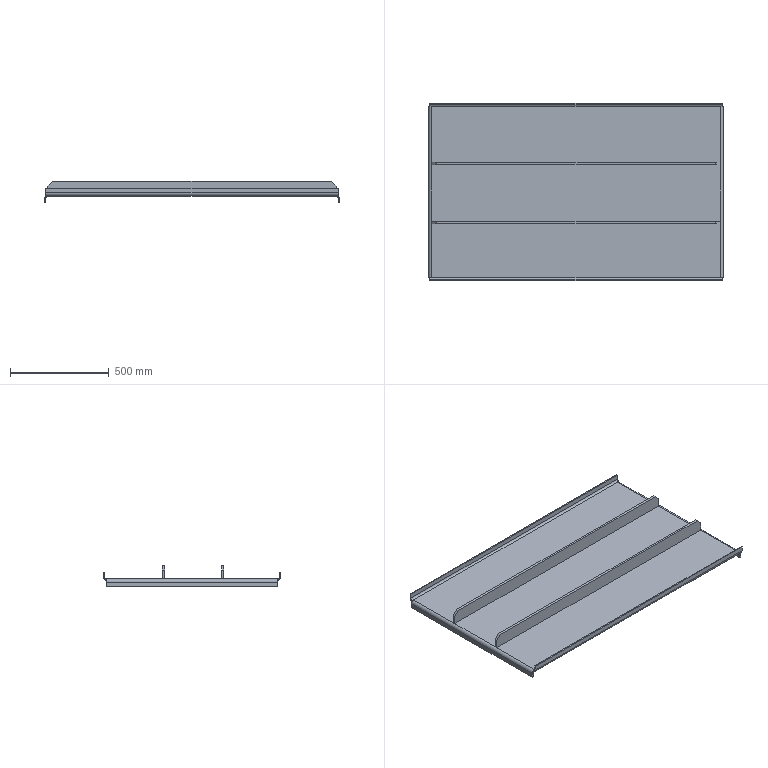Part | SolidWorks | features Chamfer 2, EdgeFlange 2, BossThin 1, FlatPattern 1, SMBaseFlange 1, SheetMetal 1, WeldmentFeature 1 | 3 solids | 58 faces | box 1492 x 898 x 110 mm | volume 11274482 mm3 | plane 50 | cylinder 8 | commonest cylinder face diameters 20 x4 32 x4
STEP:
#1=CARTESIAN_POINT('',(740.,-433.,0.));
#2=VERTEX_POINT('',#1);
#3=CARTESIAN_POINT('',(740.,-433.,-3.51));
#4=VERTEX_POINT('',#3);
#5=CARTESIAN_POINT('',(740.,-433.,0.));
#6=DIRECTION('',(0.,0.,-1.));
#7=VECTOR('',#6,1000.);
#8=LINE('',#5,#7);
#9=EDGE_CURVE('',#2,#4,#8,.T.);
#10=ORIENTED_EDGE('',*,*,#9,.T.);
#11=CARTESIAN_POINT('',(730.,-433.,0.));
#12=VERTEX_POINT('',#11);
#13=CARTESIAN_POINT('',(730.,-433.,-16.));
#14=DIRECTION('',(0.,-1.,0.));
#15=DIRECTION('',(0.,0.,-1.));
#16=AXIS2_PLACEMENT_3D('',#13,#14,#15);
#17=CIRCLE('',#16,16.);
#18=EDGE_CURVE('',#4,#12,#17,.T.);
#19=ORIENTED_EDGE('',*,*,#18,.T.);
#20=CARTESIAN_POINT('',(740.,-433.,0.));
#21=DIRECTION('',(-1.,0.,0.));
#22=VECTOR('',#21,1000.);
#23=LINE('',#20,#22);
#24=EDGE_CURVE('',#2,#12,#23,.T.);
#25=ORIENTED_EDGE('',*,*,#24,.F.);
#26=EDGE_LOOP('',(#10,#19,#25));
#27=FACE_OUTER_BOUND('',#26,.T.);
#28=CARTESIAN_POINT('',(740.,-433.,-6.));
#29=DIRECTION('',(0.,1.,0.));
#30=DIRECTION('',(0.,0.,1.));
#31=AXIS2_PLACEMENT_3D('',#28,#29,#30);
#32=PLANE('',#31);
#33=ADVANCED_FACE('',(#27),#32,.T.);
#34=CARTESIAN_POINT('',(730.,433.,0.));
#35=VERTEX_POINT('',#34);
#36=CARTESIAN_POINT('',(740.,433.,0.));
#37=VERTEX_POINT('',#36);
#38=CARTESIAN_POINT('',(-740.,433.,0.));
#39=DIRECTION('',(1.,0.,0.));
#40=VECTOR('',#39,1000.);
#41=LINE('',#38,#40);
#42=EDGE_CURVE('',#35,#37,#41,.T.);
#43=ORIENTED_EDGE('',*,*,#42,.F.);
#44=CARTESIAN_POINT('',(740.,433.,-3.51));
#45=VERTEX_POINT('',#44);
#46=CARTESIAN_POINT('',(730.,433.,-16.));
#47=DIRECTION('',(0.,1.,0.));
#48=DIRECTION('',(0.,0.,-1.));
#49=AXIS2_PLACEMENT_3D('',#46,#47,#48);
#50=CIRCLE('',#49,16.);
#51=EDGE_CURVE('',#35,#45,#50,.T.);
#52=ORIENTED_EDGE('',*,*,#51,.T.);
#53=CARTESIAN_POINT('',(740.,433.,0.));
#54=DIRECTION('',(0.,0.,-1.));
#55=VECTOR('',#54,1000.);
#56=LINE('',#53,#55);
#57=EDGE_CURVE('',#37,#45,#56,.T.);
#58=ORIENTED_EDGE('',*,*,#57,.F.);
#59=EDGE_LOOP('',(#43,#52,#58));
#60=FACE_OUTER_BOUND('',#59,.T.);
#61=CARTESIAN_POINT('',(730.,433.,-6.));
#62=DIRECTION('',(0.,-1.,0.));
#63=DIRECTION('',(1.,0.,0.));
#64=AXIS2_PLACEMENT_3D('',#61,#62,#63);
#65=PLANE('',#64);
#66=ADVANCED_FACE('',(#60),#65,.T.);
#67=CARTESIAN_POINT('',(-740.,433.,0.));
#68=VERTEX_POINT('',#67);
#69=CARTESIAN_POINT('',(-740.,433.,-3.51));
#70=VERTEX_POINT('',#69);
#71=CARTESIAN_POINT('',(-740.,433.,0.));
#72=DIRECTION('',(0.,0.,-1.));
#73=VECTOR('',#72,1000.);
#74=LINE('',#71,#73);
#75=EDGE_CURVE('',#68,#70,#74,.T.);
#76=ORIENTED_EDGE('',*,*,#75,.T.);
#77=CARTESIAN_POINT('',(-730.,433.,0.));
#78=VERTEX_POINT('',#77);
#79=CARTESIAN_POINT('',(-730.,433.,-16.));
#80=DIRECTION('',(0.,1.,0.));
#81=DIRECTION('',(0.,0.,1.));
#82=AXIS2_PLACEMENT_3D('',#79,#80,#81);
#83=CIRCLE('',#82,16.);
#84=EDGE_CURVE('',#70,#78,#83,.T.);
#85=ORIENTED_EDGE('',*,*,#84,.T.);
#86=CARTESIAN_POINT('',(-740.,433.,0.));
#87=DIRECTION('',(1.,0.,0.));
#88=VECTOR('',#87,1000.);
#89=LINE('',#86,#88);
#90=EDGE_CURVE('',#68,#78,#89,.T.);
#91=ORIENTED_EDGE('',*,*,#90,.F.);
#92=EDGE_LOOP('',(#76,#85,#91));
#93=FACE_OUTER_BOUND('',#92,.T.);
#94=CARTESIAN_POINT('',(-740.,433.,-6.));
#95=DIRECTION('',(0.,-1.,0.));
#96=DIRECTION('',(0.,0.,-1.));
#97=AXIS2_PLACEMENT_3D('',#94,#95,#96);
#98=PLANE('',#97);
#99=ADVANCED_FACE('',(#93),#98,.T.);
#100=CARTESIAN_POINT('',(-730.,-433.,0.));
#101=VERTEX_POINT('',#100);
#102=CARTESIAN_POINT('',(-740.,-433.,0.));
#103=VERTEX_POINT('',#102);
#104=CARTESIAN_POINT('',(740.,-433.,0.));
#105=DIRECTION('',(-1.,0.,0.));
#106=VECTOR('',#105,1000.);
#107=LINE('',#104,#106);
#108=EDGE_CURVE('',#101,#103,#107,.T.);
#109=ORIENTED_EDGE('',*,*,#108,.F.);
#110=CARTESIAN_POINT('',(-740.,-433.,-3.51));
#111=VERTEX_POINT('',#110);
#112=CARTESIAN_POINT('',(-730.,-433.,-16.));
#113=DIRECTION('',(0.,-1.,0.));
#114=DIRECTION('',(0.,0.,1.));
#115=AXIS2_PLACEMENT_3D('',#112,#113,#114);
#116=CIRCLE('',#115,16.);
#117=EDGE_CURVE('',#101,#111,#116,.T.);
#118=ORIENTED_EDGE('',*,*,#117,.T.);
#119=CARTESIAN_POINT('',(-740.,-433.,0.));
#120=DIRECTION('',(0.,0.,-1.));
#121=VECTOR('',#120,1000.);
#122=LINE('',#119,#121);
#123=EDGE_CURVE('',#103,#111,#122,.T.);
#124=ORIENTED_EDGE('',*,*,#123,.F.);
#125=EDGE_LOOP('',(#109,#118,#124));
#126=FACE_OUTER_BOUND('',#125,.T.);
#127=CARTESIAN_POINT('',(-730.,-433.,-6.));
#128=DIRECTION('',(0.,1.,0.));
#129=DIRECTION('',(0.,0.,1.));
#130=AXIS2_PLACEMENT_3D('',#127,#128,#129);
#131=PLANE('',#130);
#132=ADVANCED_FACE('',(#126),#131,.T.);
#133=CARTESIAN_POINT('',(730.,-433.,-6.));
#134=VERTEX_POINT('',#133);
#135=CARTESIAN_POINT('',(730.,433.,-6.));
#136=VERTEX_POINT('',#135);
#137=CARTESIAN_POINT('',(730.,-433.,-6.));
#138=DIRECTION('',(0.,1.,0.));
#139=VECTOR('',#138,1000.);
#140=LINE('',#137,#139);
#141=EDGE_CURVE('',#134,#136,#140,.T.);
#142=ORIENTED_EDGE('',*,*,#141,.F.);
#143=CARTESIAN_POINT('',(-730.,-433.,-6.));
#144=VERTEX_POINT('',#143);
#145=CARTESIAN_POINT('',(740.,-433.,-6.));
#146=DIRECTION('',(-1.,0.,0.));
#147=VECTOR('',#146,1000.);
#148=LINE('',#145,#147);
#149=EDGE_CURVE('',#134,#144,#148,.T.);
#150=ORIENTED_EDGE('',*,*,#149,.T.);
#151=CARTESIAN_POINT('',(-730.,433.,-6.));
#152=VERTEX_POINT('',#151);
#153=CARTESIAN_POINT('',(-730.,433.,-6.));
#154=DIRECTION('',(0.,-1.,0.));
#155=VECTOR('',#154,1000.);
#156=LINE('',#153,#155);
#157=EDGE_CURVE('',#152,#144,#156,.T.);
#158=ORIENTED_EDGE('',*,*,#157,.F.);
#159=CARTESIAN_POINT('',(-740.,433.,-6.));
#160=DIRECTION('',(1.,0.,0.));
#161=VECTOR('',#160,1000.);
#162=LINE('',#159,#161);
#163=EDGE_CURVE('',#152,#136,#162,.T.);
#164=ORIENTED_EDGE('',*,*,#163,.T.);
#165=EDGE_LOOP('',(#142,#150,#158,#164));
#166=FACE_OUTER_BOUND('',#165,.T.);
#167=CARTESIAN_POINT('',(0.,0.,-6.));
#168=DIRECTION('',(0.,0.,1.));
#169=DIRECTION('',(1.,0.,0.));
#170=AXIS2_PLACEMENT_3D('',#167,#168,#169);
#171=PLANE('',#170);
#172=ADVANCED_FACE('',(#166),#171,.F.);
#173=CARTESIAN_POINT('',(740.,-433.,0.));
#174=DIRECTION('',(-1.,0.,0.));
#175=VECTOR('',#174,1000.);
#176=LINE('',#173,#175);
#177=EDGE_CURVE('',#12,#101,#176,.T.);
#178=ORIENTED_EDGE('',*,*,#177,.F.);
#179=CARTESIAN_POINT('',(730.,-433.,0.));
#180=DIRECTION('',(0.,1.,0.));
#181=VECTOR('',#180,1000.);
#182=LINE('',#179,#181);
#183=EDGE_CURVE('',#12,#35,#182,.T.);
#184=ORIENTED_EDGE('',*,*,#183,.T.);
#185=CARTESIAN_POINT('',(-740.,433.,0.));
#186=DIRECTION('',(1.,0.,0.));
#187=VECTOR('',#186,1000.);
#188=LINE('',#185,#187);
#189=EDGE_CURVE('',#78,#35,#188,.T.);
#190=ORIENTED_EDGE('',*,*,#189,.F.);
#191=CARTESIAN_POINT('',(-730.,433.,0.));
#192=DIRECTION('',(0.,-1.,0.));
#193=VECTOR('',#192,1000.);
#194=LINE('',#191,#193);
#195=EDGE_CURVE('',#78,#101,#194,.T.);
#196=ORIENTED_EDGE('',*,*,#195,.T.);
#197=EDGE_LOOP('',(#178,#184,#190,#196));
#198=FACE_OUTER_BOUND('',#197,.T.);
#199=CARTESIAN_POINT('',(0.,0.,0.));
#200=DIRECTION('',(0.,0.,1.));
#201=DIRECTION('',(1.,0.,0.));
#202=AXIS2_PLACEMENT_3D('',#199,#200,#201);
#203=PLANE('',#202);
#204=ADVANCED_FACE('',(#198),#203,.T.);
#205=CARTESIAN_POINT('',(740.,443.,10.));
#206=VERTEX_POINT('',#205);
#207=CARTESIAN_POINT('',(740.,449.,10.));
#208=VERTEX_POINT('',#207);
#209=CARTESIAN_POINT('',(740.,449.,10.));
#210=DIRECTION('',(0.,1.,0.));
#211=VECTOR('',#210,1000.);
#212=LINE('',#209,#211);
#213=EDGE_CURVE('',#206,#208,#212,.T.);
#214=ORIENTED_EDGE('',*,*,#213,.F.);
#215=CARTESIAN_POINT('',(740.,433.,10.));
#216=DIRECTION('',(1.,0.,0.));
#217=DIRECTION('',(0.,0.,1.));
#218=AXIS2_PLACEMENT_3D('',#215,#216,#217);
#219=CIRCLE('',#218,10.);
#220=EDGE_CURVE('',#37,#206,#219,.T.);
#221=ORIENTED_EDGE('',*,*,#220,.F.);
#222=ORIENTED_EDGE('',*,*,#57,.T.);
#223=CARTESIAN_POINT('',(740.,433.,-6.));
#224=VERTEX_POINT('',#223);
#225=CARTESIAN_POINT('',(740.,433.,0.));
#226=DIRECTION('',(0.,0.,-1.));
#227=VECTOR('',#226,1000.);
#228=LINE('',#225,#227);
#229=EDGE_CURVE('',#45,#224,#228,.T.);
#230=ORIENTED_EDGE('',*,*,#229,.T.);
#231=CARTESIAN_POINT('',(740.,433.,10.));
#232=DIRECTION('',(1.,0.,0.));
#233=DIRECTION('',(0.,0.,1.));
#234=AXIS2_PLACEMENT_3D('',#231,#232,#233);
#235=CIRCLE('',#234,16.);
#236=EDGE_CURVE('',#224,#208,#235,.T.);
#237=ORIENTED_EDGE('',*,*,#236,.T.);
#238=EDGE_LOOP('',(#214,#221,#222,#230,#237));
#239=FACE_OUTER_BOUND('',#238,.T.);
#240=CARTESIAN_POINT('',(740.,433.,10.));
#241=DIRECTION('',(1.,0.,0.));
#242=DIRECTION('',(0.,0.,-1.));
#243=AXIS2_PLACEMENT_3D('',#240,#241,#242);
#244=PLANE('',#243);
#245=ADVANCED_FACE('',(#239),#244,.T.);
#246=CARTESIAN_POINT('',(-740.,443.,10.));
#247=VERTEX_POINT('',#246);
#248=CARTESIAN_POINT('',(-740.,433.,10.));
#249=DIRECTION('',(-1.,0.,0.));
#250=DIRECTION('',(0.,0.,1.));
#251=AXIS2_PLACEMENT_3D('',#248,#249,#250);
#252=CIRCLE('',#251,10.);
#253=EDGE_CURVE('',#247,#68,#252,.T.);
#254=ORIENTED_EDGE('',*,*,#253,.F.);
#255=CARTESIAN_POINT('',(-740.,449.,10.));
#256=VERTEX_POINT('',#255);
#257=CARTESIAN_POINT('',(-740.,443.,10.));
#258=DIRECTION('',(0.,1.,0.));
#259=VECTOR('',#258,1000.);
#260=LINE('',#257,#259);
#261=EDGE_CURVE('',#247,#256,#260,.T.);
#262=ORIENTED_EDGE('',*,*,#261,.T.);
#263=CARTESIAN_POINT('',(-740.,433.,-6.));
#264=VERTEX_POINT('',#263);
#265=CARTESIAN_POINT('',(-740.,433.,10.));
#266=DIRECTION('',(-1.,0.,0.));
#267=DIRECTION('',(0.,0.,1.));
#268=AXIS2_PLACEMENT_3D('',#265,#266,#267);
#269=CIRCLE('',#268,16.);
#270=EDGE_CURVE('',#256,#264,#269,.T.);
#271=ORIENTED_EDGE('',*,*,#270,.T.);
#272=CARTESIAN_POINT('',(-740.,433.,0.));
#273=DIRECTION('',(0.,0.,-1.));
#274=VECTOR('',#273,1000.);
#275=LINE('',#272,#274);
#276=EDGE_CURVE('',#70,#264,#275,.T.);
#277=ORIENTED_EDGE('',*,*,#276,.F.);
#278=ORIENTED_EDGE('',*,*,#75,.F.);
#279=EDGE_LOOP('',(#254,#262,#271,#277,#278));
#280=FACE_OUTER_BOUND('',#279,.T.);
#281=CARTESIAN_POINT('',(-740.,433.,10.));
#282=DIRECTION('',(1.,0.,0.));
#283=DIRECTION('',(0.,0.,-1.));
#284=AXIS2_PLACEMENT_3D('',#281,#282,#283);
#285=PLANE('',#284);
#286=ADVANCED_FACE('',(#280),#285,.F.);
#287=CARTESIAN_POINT('',(-740.,433.,-6.));
#288=DIRECTION('',(1.,0.,0.));
#289=VECTOR('',#288,1000.);
#290=LINE('',#287,#289);
#291=EDGE_CURVE('',#264,#152,#290,.T.);
#292=ORIENTED_EDGE('',*,*,#291,.F.);
#293=ORIENTED_EDGE('',*,*,#270,.F.);
#294=CARTESIAN_POINT('',(740.,449.,10.));
#295=DIRECTION('',(1.,0.,0.));
#296=VECTOR('',#295,1000.);
#297=LINE('',#294,#296);
#298=EDGE_CURVE('',#256,#208,#297,.T.);
#299=ORIENTED_EDGE('',*,*,#298,.T.);
#300=ORIENTED_EDGE('',*,*,#236,.F.);
#301=CARTESIAN_POINT('',(730.,433.,-6.));
#302=DIRECTION('',(1.,0.,0.));
#303=VECTOR('',#302,1000.);
#304=LINE('',#301,#303);
#305=EDGE_CURVE('',#136,#224,#304,.T.);
#306=ORIENTED_EDGE('',*,*,#305,.F.);
#307=ORIENTED_EDGE('',*,*,#163,.F.);
#308=EDGE_LOOP('',(#292,#293,#299,#300,#306,#307));
#309=FACE_OUTER_BOUND('',#308,.T.);
#310=CARTESIAN_POINT('',(-740.,433.,10.));
#311=DIRECTION('',(-1.,0.,0.));
#312=DIRECTION('',(0.,1.,0.));
#313=AXIS2_PLACEMENT_3D('',#310,#311,#312);
#314=CYLINDRICAL_SURFACE('',#313,16.);
#315=ADVANCED_FACE('',(#309),#314,.T.);
#316=ORIENTED_EDGE('',*,*,#90,.T.);
#317=ORIENTED_EDGE('',*,*,#189,.T.);
#318=ORIENTED_EDGE('',*,*,#42,.T.);
#319=ORIENTED_EDGE('',*,*,#220,.T.);
#320=CARTESIAN_POINT('',(740.,443.,10.));
#321=DIRECTION('',(-1.,0.,0.));
#322=VECTOR('',#321,1000.);
#323=LINE('',#320,#322);
#324=EDGE_CURVE('',#206,#247,#323,.T.);
#325=ORIENTED_EDGE('',*,*,#324,.T.);
#326=ORIENTED_EDGE('',*,*,#253,.T.);
#327=EDGE_LOOP('',(#316,#317,#318,#319,#325,#326));
#328=FACE_OUTER_BOUND('',#327,.T.);
#329=CARTESIAN_POINT('',(-740.,433.,10.));
#330=DIRECTION('',(-1.,0.,0.));
#331=DIRECTION('',(0.,1.,0.));
#332=AXIS2_PLACEMENT_3D('',#329,#330,#331);
#333=CYLINDRICAL_SURFACE('',#332,10.);
#334=ADVANCED_FACE('',(#328),#333,.F.);
#335=ORIENTED_EDGE('',*,*,#213,.T.);
#336=CARTESIAN_POINT('',(740.,449.,34.));
#337=VERTEX_POINT('',#336);
#338=CARTESIAN_POINT('',(740.,449.,0.));
#339=DIRECTION('',(0.,0.,-1.));
#340=VECTOR('',#339,1000.);
#341=LINE('',#338,#340);
#342=EDGE_CURVE('',#337,#208,#341,.T.);
#343=ORIENTED_EDGE('',*,*,#342,.F.);
#344=CARTESIAN_POINT('',(740.,443.,34.));
#345=VERTEX_POINT('',#344);
#346=CARTESIAN_POINT('',(740.,449.,34.));
#347=DIRECTION('',(0.,-1.,0.));
#348=VECTOR('',#347,1000.);
#349=LINE('',#346,#348);
#350=EDGE_CURVE('',#337,#345,#349,.T.);
#351=ORIENTED_EDGE('',*,*,#350,.T.);
#352=CARTESIAN_POINT('',(740.,443.,0.));
#353=DIRECTION('',(0.,0.,-1.));
#354=VECTOR('',#353,1000.);
#355=LINE('',#352,#354);
#356=EDGE_CURVE('',#345,#206,#355,.T.);
#357=ORIENTED_EDGE('',*,*,#356,.T.);
#358=EDGE_LOOP('',(#335,#343,#351,#357));
#359=FACE_OUTER_BOUND('',#358,.T.);
#360=CARTESIAN_POINT('',(740.,449.,0.));
#361=DIRECTION('',(-1.,0.,0.));
#362=DIRECTION('',(0.,0.,1.));
#363=AXIS2_PLACEMENT_3D('',#360,#361,#362);
#364=PLANE('',#363);
#365=ADVANCED_FACE('',(#359),#364,.F.);
#366=ORIENTED_EDGE('',*,*,#261,.F.);
#367=CARTESIAN_POINT('',(-740.,443.,34.));
#368=VERTEX_POINT('',#367);
#369=CARTESIAN_POINT('',(-740.,443.,34.));
#370=DIRECTION('',(0.,0.,1.));
#371=VECTOR('',#370,1000.);
#372=LINE('',#369,#371);
#373=EDGE_CURVE('',#247,#368,#372,.T.);
#374=ORIENTED_EDGE('',*,*,#373,.T.);
#375=CARTESIAN_POINT('',(-740.,449.,34.));
#376=VERTEX_POINT('',#375);
#377=CARTESIAN_POINT('',(-740.,449.,34.));
#378=DIRECTION('',(0.,-1.,0.));
#379=VECTOR('',#378,1000.);
#380=LINE('',#377,#379);
#381=EDGE_CURVE('',#376,#368,#380,.T.);
#382=ORIENTED_EDGE('',*,*,#381,.F.);
#383=CARTESIAN_POINT('',(-740.,449.,0.));
#384=DIRECTION('',(0.,0.,1.));
#385=VECTOR('',#384,1000.);
#386=LINE('',#383,#385);
#387=EDGE_CURVE('',#256,#376,#386,.T.);
#388=ORIENTED_EDGE('',*,*,#387,.F.);
#389=EDGE_LOOP('',(#366,#374,#382,#388));
#390=FACE_OUTER_BOUND('',#389,.T.);
#391=CARTESIAN_POINT('',(-740.,449.,34.));
#392=DIRECTION('',(1.,0.,0.));
#393=DIRECTION('',(0.,0.,-1.));
#394=AXIS2_PLACEMENT_3D('',#391,#392,#393);
#395=PLANE('',#394);
#396=ADVANCED_FACE('',(#390),#395,.F.);
#397=ORIENTED_EDGE('',*,*,#298,.F.);
#398=ORIENTED_EDGE('',*,*,#387,.T.);
#399=CARTESIAN_POINT('',(0.,449.,34.));
#400=DIRECTION('',(1.,0.,0.));
#401=VECTOR('',#400,1000.);
#402=LINE('',#399,#401);
#403=EDGE_CURVE('',#376,#337,#402,.T.);
#404=ORIENTED_EDGE('',*,*,#403,.T.);
#405=ORIENTED_EDGE('',*,*,#342,.T.);
#406=EDGE_LOOP('',(#397,#398,#404,#405));
#407=FACE_OUTER_BOUND('',#406,.T.);
#408=CARTESIAN_POINT('',(0.,449.,0.));
#409=DIRECTION('',(0.,-1.,0.));
#410=DIRECTION('',(0.,0.,-1.));
#411=AXIS2_PLACEMENT_3D('',#408,#409,#410);
#412=PLANE('',#411);
#413=ADVANCED_FACE('',(#407),#412,.F.);
#414=ORIENTED_EDGE('',*,*,#373,.F.);
#415=ORIENTED_EDGE('',*,*,#324,.F.);
#416=ORIENTED_EDGE('',*,*,#356,.F.);
#417=CARTESIAN_POINT('',(740.,443.,34.));
#418=DIRECTION('',(1.,0.,0.));
#419=VECTOR('',#418,1000.);
#420=LINE('',#417,#419);
#421=EDGE_CURVE('',#368,#345,#420,.T.);
#422=ORIENTED_EDGE('',*,*,#421,.F.);
#423=EDGE_LOOP('',(#414,#415,#416,#422));
#424=FACE_OUTER_BOUND('',#423,.T.);
#425=CARTESIAN_POINT('',(0.,443.,0.));
#426=DIRECTION('',(0.,-1.,0.));
#427=DIRECTION('',(0.,0.,-1.));
#428=AXIS2_PLACEMENT_3D('',#425,#426,#427);
#429=PLANE('',#428);
#430=ADVANCED_FACE('',(#424),#429,.T.);
#431=ORIENTED_EDGE('',*,*,#421,.T.);
#432=ORIENTED_EDGE('',*,*,#350,.F.);
#433=ORIENTED_EDGE('',*,*,#403,.F.);
#434=ORIENTED_EDGE('',*,*,#381,.T.);
#435=EDGE_LOOP('',(#431,#432,#433,#434));
#436=FACE_OUTER_BOUND('',#435,.T.);
#437=CARTESIAN_POINT('',(740.,449.,34.));
#438=DIRECTION('',(0.,0.,-1.));
#439=DIRECTION('',(0.,1.,0.));
#440=AXIS2_PLACEMENT_3D('',#437,#438,#439);
#441=PLANE('',#440);
#442=ADVANCED_FACE('',(#436),#441,.F.);
#443=CARTESIAN_POINT('',(-740.,-443.,10.));
#444=VERTEX_POINT('',#443);
#445=CARTESIAN_POINT('',(-740.,-449.,10.));
#446=VERTEX_POINT('',#445);
#447=CARTESIAN_POINT('',(-740.,-449.,10.));
#448=DIRECTION('',(0.,-1.,0.));
#449=VECTOR('',#448,1000.);
#450=LINE('',#447,#449);
#451=EDGE_CURVE('',#444,#446,#450,.T.);
#452=ORIENTED_EDGE('',*,*,#451,.F.);
#453=CARTESIAN_POINT('',(-740.,-433.,10.));
#454=DIRECTION('',(-1.,0.,0.));
#455=DIRECTION('',(0.,0.,-1.));
#456=AXIS2_PLACEMENT_3D('',#453,#454,#455);
#457=CIRCLE('',#456,10.);
#458=EDGE_CURVE('',#103,#444,#457,.T.);
#459=ORIENTED_EDGE('',*,*,#458,.F.);
#460=ORIENTED_EDGE('',*,*,#123,.T.);
#461=CARTESIAN_POINT('',(-740.,-433.,-6.));
#462=VERTEX_POINT('',#461);
#463=CARTESIAN_POINT('',(-740.,-433.,0.));
#464=DIRECTION('',(0.,0.,-1.));
#465=VECTOR('',#464,1000.);
#466=LINE('',#463,#465);
#467=EDGE_CURVE('',#111,#462,#466,.T.);
#468=ORIENTED_EDGE('',*,*,#467,.T.);
#469=CARTESIAN_POINT('',(-740.,-433.,10.));
#470=DIRECTION('',(-1.,0.,0.));
#471=DIRECTION('',(0.,0.,-1.));
#472=AXIS2_PLACEMENT_3D('',#469,#470,#471);
#473=CIRCLE('',#472,16.);
#474=EDGE_CURVE('',#462,#446,#473,.T.);
#475=ORIENTED_EDGE('',*,*,#474,.T.);
#476=EDGE_LOOP('',(#452,#459,#460,#468,#475));
#477=FACE_OUTER_BOUND('',#476,.T.);
#478=CARTESIAN_POINT('',(-740.,-433.,10.));
#479=DIRECTION('',(-1.,0.,0.));
#480=DIRECTION('',(0.,0.,1.));
#481=AXIS2_PLACEMENT_3D('',#478,#479,#480);
#482=PLANE('',#481);
#483=ADVANCED_FACE('',(#477),#482,.T.);
#484=CARTESIAN_POINT('',(740.,-443.,10.));
#485=VERTEX_POINT('',#484);
#486=CARTESIAN_POINT('',(740.,-433.,10.));
#487=DIRECTION('',(1.,0.,0.));
#488=DIRECTION('',(0.,0.,-1.));
#489=AXIS2_PLACEMENT_3D('',#486,#487,#488);
#490=CIRCLE('',#489,10.);
#491=EDGE_CURVE('',#485,#2,#490,.T.);
#492=ORIENTED_EDGE('',*,*,#491,.F.);
#493=CARTESIAN_POINT('',(740.,-449.,10.));
#494=VERTEX_POINT('',#493);
#495=CARTESIAN_POINT('',(740.,-443.,10.));
#496=DIRECTION('',(0.,-1.,0.));
#497=VECTOR('',#496,1000.);
#498=LINE('',#495,#497);
#499=EDGE_CURVE('',#485,#494,#498,.T.);
#500=ORIENTED_EDGE('',*,*,#499,.T.);
#501=CARTESIAN_POINT('',(740.,-433.,-6.));
#502=VERTEX_POINT('',#501);
#503=CARTESIAN_POINT('',(740.,-433.,10.));
#504=DIRECTION('',(1.,0.,0.));
#505=DIRECTION('',(0.,0.,-1.));
#506=AXIS2_PLACEMENT_3D('',#503,#504,#505);
#507=CIRCLE('',#506,16.);
#508=EDGE_CURVE('',#494,#502,#507,.T.);
#509=ORIENTED_EDGE('',*,*,#508,.T.);
#510=CARTESIAN_POINT('',(740.,-433.,0.));
#511=DIRECTION('',(0.,0.,-1.));
#512=VECTOR('',#511,1000.);
#513=LINE('',#510,#512);
#514=EDGE_CURVE('',#4,#502,#513,.T.);
#515=ORIENTED_EDGE('',*,*,#514,.F.);
#516=ORIENTED_EDGE('',*,*,#9,.F.);
#517=EDGE_LOOP('',(#492,#500,#509,#515,#516));
#518=FACE_OUTER_BOUND('',#517,.T.);
#519=CARTESIAN_POINT('',(740.,-433.,10.));
#520=DIRECTION('',(-1.,0.,0.));
#521=DIRECTION('',(0.,0.,1.));
#522=AXIS2_PLACEMENT_3D('',#519,#520,#521);
#523=PLANE('',#522);
#524=ADVANCED_FACE('',(#518),#523,.F.);
#525=CARTESIAN_POINT('',(740.,-433.,-6.));
#526=DIRECTION('',(-1.,0.,0.));
#527=VECTOR('',#526,1000.);
#528=LINE('',#525,#527);
#529=EDGE_CURVE('',#502,#134,#528,.T.);
#530=ORIENTED_EDGE('',*,*,#529,.F.);
#531=ORIENTED_EDGE('',*,*,#508,.F.);
#532=CARTESIAN_POINT('',(-740.,-449.,10.));
#533=DIRECTION('',(-1.,0.,0.));
#534=VECTOR('',#533,1000.);
#535=LINE('',#532,#534);
#536=EDGE_CURVE('',#494,#446,#535,.T.);
#537=ORIENTED_EDGE('',*,*,#536,.T.);
#538=ORIENTED_EDGE('',*,*,#474,.F.);
#539=CARTESIAN_POINT('',(-730.,-433.,-6.));
#540=DIRECTION('',(-1.,0.,0.));
#541=VECTOR('',#540,1000.);
#542=LINE('',#539,#541);
#543=EDGE_CURVE('',#144,#462,#542,.T.);
#544=ORIENTED_EDGE('',*,*,#543,.F.);
#545=ORIENTED_EDGE('',*,*,#149,.F.);
#546=EDGE_LOOP('',(#530,#531,#537,#538,#544,#545));
#547=FACE_OUTER_BOUND('',#546,.T.);
#548=CARTESIAN_POINT('',(740.,-433.,10.));
#549=DIRECTION('',(1.,0.,0.));
#550=DIRECTION('',(0.,-1.,0.));
#551=AXIS2_PLACEMENT_3D('',#548,#549,#550);
#552=CYLINDRICAL_SURFACE('',#551,16.);
#553=ADVANCED_FACE('',(#547),#552,.T.);
#554=ORIENTED_EDGE('',*,*,#24,.T.);
#555=ORIENTED_EDGE('',*,*,#177,.T.);
#556=ORIENTED_EDGE('',*,*,#108,.T.);
#557=ORIENTED_EDGE('',*,*,#458,.T.);
#558=CARTESIAN_POINT('',(-740.,-443.,10.));
#559=DIRECTION('',(1.,0.,0.));
#560=VECTOR('',#559,1000.);
#561=LINE('',#558,#560);
#562=EDGE_CURVE('',#444,#485,#561,.T.);
#563=ORIENTED_EDGE('',*,*,#562,.T.);
#564=ORIENTED_EDGE('',*,*,#491,.T.);
#565=EDGE_LOOP('',(#554,#555,#556,#557,#563,#564));
#566=FACE_OUTER_BOUND('',#565,.T.);
#567=CARTESIAN_POINT('',(740.,-433.,10.));
#568=DIRECTION('',(1.,0.,0.));
#569=DIRECTION('',(0.,-1.,0.));
#570=AXIS2_PLACEMENT_3D('',#567,#568,#569);
#571=CYLINDRICAL_SURFACE('',#570,10.);
#572=ADVANCED_FACE('',(#566),#571,.F.);
#573=ORIENTED_EDGE('',*,*,#451,.T.);
#574=CARTESIAN_POINT('',(-740.,-449.,34.));
#575=VERTEX_POINT('',#574);
#576=CARTESIAN_POINT('',(-740.,-449.,0.));
#577=DIRECTION('',(0.,0.,-1.));
#578=VECTOR('',#577,1000.);
#579=LINE('',#576,#578);
#580=EDGE_CURVE('',#575,#446,#579,.T.);
#581=ORIENTED_EDGE('',*,*,#580,.F.);
#582=CARTESIAN_POINT('',(-740.,-443.,34.));
#583=VERTEX_POINT('',#582);
#584=CARTESIAN_POINT('',(-740.,-449.,34.));
#585=DIRECTION('',(0.,1.,0.));
#586=VECTOR('',#585,1000.);
#587=LINE('',#584,#586);
#588=EDGE_CURVE('',#575,#583,#587,.T.);
#589=ORIENTED_EDGE('',*,*,#588,.T.);
#590=CARTESIAN_POINT('',(-740.,-443.,0.));
#591=DIRECTION('',(0.,0.,-1.));
#592=VECTOR('',#591,1000.);
#593=LINE('',#590,#592);
#594=EDGE_CURVE('',#583,#444,#593,.T.);
#595=ORIENTED_EDGE('',*,*,#594,.T.);
#596=EDGE_LOOP('',(#573,#581,#589,#595));
#597=FACE_OUTER_BOUND('',#596,.T.);
#598=CARTESIAN_POINT('',(-740.,-449.,0.));
#599=DIRECTION('',(1.,0.,0.));
#600=DIRECTION('',(0.,0.,-1.));
#601=AXIS2_PLACEMENT_3D('',#598,#599,#600);
#602=PLANE('',#601);
#603=ADVANCED_FACE('',(#597),#602,.F.);
#604=ORIENTED_EDGE('',*,*,#499,.F.);
#605=CARTESIAN_POINT('',(740.,-443.,34.));
#606=VERTEX_POINT('',#605);
#607=CARTESIAN_POINT('',(740.,-443.,34.));
#608=DIRECTION('',(0.,0.,1.));
#609=VECTOR('',#608,1000.);
#610=LINE('',#607,#609);
#611=EDGE_CURVE('',#485,#606,#610,.T.);
#612=ORIENTED_EDGE('',*,*,#611,.T.);
#613=CARTESIAN_POINT('',(740.,-449.,34.));
#614=VERTEX_POINT('',#613);
#615=CARTESIAN_POINT('',(740.,-449.,34.));
#616=DIRECTION('',(0.,1.,0.));
#617=VECTOR('',#616,1000.);
#618=LINE('',#615,#617);
#619=EDGE_CURVE('',#614,#606,#618,.T.);
#620=ORIENTED_EDGE('',*,*,#619,.F.);
#621=CARTESIAN_POINT('',(740.,-449.,0.));
#622=DIRECTION('',(0.,0.,1.));
#623=VECTOR('',#622,1000.);
#624=LINE('',#621,#623);
#625=EDGE_CURVE('',#494,#614,#624,.T.);
#626=ORIENTED_EDGE('',*,*,#625,.F.);
#627=EDGE_LOOP('',(#604,#612,#620,#626));
#628=FACE_OUTER_BOUND('',#627,.T.);
#629=CARTESIAN_POINT('',(740.,-449.,34.));
#630=DIRECTION('',(-1.,0.,0.));
#631=DIRECTION('',(0.,0.,1.));
#632=AXIS2_PLACEMENT_3D('',#629,#630,#631);
#633=PLANE('',#632);
#634=ADVANCED_FACE('',(#628),#633,.F.);
#635=ORIENTED_EDGE('',*,*,#536,.F.);
#636=ORIENTED_EDGE('',*,*,#625,.T.);
#637=CARTESIAN_POINT('',(0.,-449.,34.));
#638=DIRECTION('',(-1.,0.,0.));
#639=VECTOR('',#638,1000.);
#640=LINE('',#637,#639);
#641=EDGE_CURVE('',#614,#575,#640,.T.);
#642=ORIENTED_EDGE('',*,*,#641,.T.);
#643=ORIENTED_EDGE('',*,*,#580,.T.);
#644=EDGE_LOOP('',(#635,#636,#642,#643));
#645=FACE_OUTER_BOUND('',#644,.T.);
#646=CARTESIAN_POINT('',(0.,-449.,0.));
#647=DIRECTION('',(0.,1.,0.));
#648=DIRECTION('',(0.,0.,1.));
#649=AXIS2_PLACEMENT_3D('',#646,#647,#648);
#650=PLANE('',#649);
#651=ADVANCED_FACE('',(#645),#650,.F.);
#652=ORIENTED_EDGE('',*,*,#611,.F.);
#653=ORIENTED_EDGE('',*,*,#562,.F.);
#654=ORIENTED_EDGE('',*,*,#594,.F.);
#655=CARTESIAN_POINT('',(-740.,-443.,34.));
#656=DIRECTION('',(-1.,0.,0.));
#657=VECTOR('',#656,1000.);
#658=LINE('',#655,#657);
#659=EDGE_CURVE('',#606,#583,#658,.T.);
#660=ORIENTED_EDGE('',*,*,#659,.F.);
#661=EDGE_LOOP('',(#652,#653,#654,#660));
#662=FACE_OUTER_BOUND('',#661,.T.);
#663=CARTESIAN_POINT('',(0.,-443.,0.));
#664=DIRECTION('',(0.,1.,0.));
#665=DIRECTION('',(0.,0.,1.));
#666=AXIS2_PLACEMENT_3D('',#663,#664,#665);
#667=PLANE('',#666);
#668=ADVANCED_FACE('',(#662),#667,.T.);
#669=ORIENTED_EDGE('',*,*,#659,.T.);
#670=ORIENTED_EDGE('',*,*,#588,.F.);
#671=ORIENTED_EDGE('',*,*,#641,.F.);
#672=ORIENTED_EDGE('',*,*,#619,.T.);
#673=EDGE_LOOP('',(#669,#670,#671,#672));
#674=FACE_OUTER_BOUND('',#673,.T.);
#675=CARTESIAN_POINT('',(-740.,-449.,34.));
#676=DIRECTION('',(0.,0.,-1.));
#677=DIRECTION('',(0.,1.,0.));
#678=AXIS2_PLACEMENT_3D('',#675,#676,#677);
#679=PLANE('',#678);
#680=ADVANCED_FACE('',(#674),#679,.F.);
#681=ORIENTED_EDGE('',*,*,#467,.F.);
#682=CARTESIAN_POINT('',(-746.,-433.,-16.));
#683=VERTEX_POINT('',#682);
#684=CARTESIAN_POINT('',(-730.,-433.,-16.));
#685=DIRECTION('',(0.,-1.,0.));
#686=DIRECTION('',(0.,0.,1.));
#687=AXIS2_PLACEMENT_3D('',#684,#685,#686);
#688=CIRCLE('',#687,16.);
#689=EDGE_CURVE('',#111,#683,#688,.T.);
#690=ORIENTED_EDGE('',*,*,#689,.T.);
#691=CARTESIAN_POINT('',(-740.,-433.,-16.));
#692=VERTEX_POINT('',#691);
#693=CARTESIAN_POINT('',(-740.,-433.,-16.));
#694=DIRECTION('',(-1.,0.,0.));
#695=VECTOR('',#694,1000.);
#696=LINE('',#693,#695);
#697=EDGE_CURVE('',#692,#683,#696,.T.);
#698=ORIENTED_EDGE('',*,*,#697,.F.);
#699=CARTESIAN_POINT('',(-730.,-433.,-16.));
#700=DIRECTION('',(0.,-1.,0.));
#701=DIRECTION('',(0.,0.,1.));
#702=AXIS2_PLACEMENT_3D('',#699,#700,#701);
#703=CIRCLE('',#702,10.);
#704=EDGE_CURVE('',#144,#692,#703,.T.);
#705=ORIENTED_EDGE('',*,*,#704,.F.);
#706=ORIENTED_EDGE('',*,*,#543,.T.);
#707=EDGE_LOOP('',(#681,#690,#698,#705,#706));
#708=FACE_OUTER_BOUND('',#707,.T.);
#709=CARTESIAN_POINT('',(-730.,-433.,-16.));
#710=DIRECTION('',(0.,-1.,0.));
#711=DIRECTION('',(0.,0.,-1.));
#712=AXIS2_PLACEMENT_3D('',#709,#710,#711);
#713=PLANE('',#712);
#714=ADVANCED_FACE('',(#708),#713,.T.);
#715=CARTESIAN_POINT('',(-746.,433.,-16.));
#716=VERTEX_POINT('',#715);
#717=CARTESIAN_POINT('',(-730.,433.,-16.));
#718=DIRECTION('',(0.,1.,0.));
#719=DIRECTION('',(0.,0.,1.));
#720=AXIS2_PLACEMENT_3D('',#717,#718,#719);
#721=CIRCLE('',#720,16.);
#722=EDGE_CURVE('',#716,#70,#721,.T.);
#723=ORIENTED_EDGE('',*,*,#722,.T.);
#724=ORIENTED_EDGE('',*,*,#276,.T.);
#725=ORIENTED_EDGE('',*,*,#291,.T.);
#726=CARTESIAN_POINT('',(-740.,433.,-16.));
#727=VERTEX_POINT('',#726);
#728=CARTESIAN_POINT('',(-730.,433.,-16.));
#729=DIRECTION('',(0.,1.,0.));
#730=DIRECTION('',(0.,0.,1.));
#731=AXIS2_PLACEMENT_3D('',#728,#729,#730);
#732=CIRCLE('',#731,10.);
#733=EDGE_CURVE('',#727,#152,#732,.T.);
#734=ORIENTED_EDGE('',*,*,#733,.F.);
#735=CARTESIAN_POINT('',(-740.,433.,-16.));
#736=DIRECTION('',(-1.,0.,0.));
#737=VECTOR('',#736,1000.);
#738=LINE('',#735,#737);
#739=EDGE_CURVE('',#727,#716,#738,.T.);
#740=ORIENTED_EDGE('',*,*,#739,.T.);
#741=EDGE_LOOP('',(#723,#724,#725,#734,#740));
#742=FACE_OUTER_BOUND('',#741,.T.);
#743=CARTESIAN_POINT('',(-730.,433.,-16.));
#744=DIRECTION('',(0.,-1.,0.));
#745=DIRECTION('',(0.,0.,-1.));
#746=AXIS2_PLACEMENT_3D('',#743,#744,#745);
#747=PLANE('',#746);
#748=ADVANCED_FACE('',(#742),#747,.F.);
#749=ORIENTED_EDGE('',*,*,#195,.F.);
#750=ORIENTED_EDGE('',*,*,#84,.F.);
#751=ORIENTED_EDGE('',*,*,#722,.F.);
#752=CARTESIAN_POINT('',(-746.,0.,-16.));
#753=DIRECTION('',(0.,1.,0.));
#754=VECTOR('',#753,1000.);
#755=LINE('',#752,#754);
#756=EDGE_CURVE('',#683,#716,#755,.T.);
#757=ORIENTED_EDGE('',*,*,#756,.F.);
#758=ORIENTED_EDGE('',*,*,#689,.F.);
#759=ORIENTED_EDGE('',*,*,#117,.F.);
#760=EDGE_LOOP('',(#749,#750,#751,#757,#758,#759));
#761=FACE_OUTER_BOUND('',#760,.T.);
#762=CARTESIAN_POINT('',(-730.,433.,-16.));
#763=DIRECTION('',(0.,1.,0.));
#764=DIRECTION('',(-1.,0.,0.));
#765=AXIS2_PLACEMENT_3D('',#762,#763,#764);
#766=CYLINDRICAL_SURFACE('',#765,16.);
#767=ADVANCED_FACE('',(#761),#766,.T.);
#768=ORIENTED_EDGE('',*,*,#157,.T.);
#769=ORIENTED_EDGE('',*,*,#704,.T.);
#770=CARTESIAN_POINT('',(-740.,-433.,-16.));
#771=DIRECTION('',(0.,1.,0.));
#772=VECTOR('',#771,1000.);
#773=LINE('',#770,#772);
#774=EDGE_CURVE('',#692,#727,#773,.T.);
#775=ORIENTED_EDGE('',*,*,#774,.T.);
#776=ORIENTED_EDGE('',*,*,#733,.T.);
#777=EDGE_LOOP('',(#768,#769,#775,#776));
#778=FACE_OUTER_BOUND('',#777,.T.);
#779=CARTESIAN_POINT('',(-730.,433.,-16.));
#780=DIRECTION('',(0.,1.,0.));
#781=DIRECTION('',(-1.,0.,0.));
#782=AXIS2_PLACEMENT_3D('',#779,#780,#781);
#783=CYLINDRICAL_SURFACE('',#782,10.);
#784=ADVANCED_FACE('',(#778),#783,.F.);
#785=CARTESIAN_POINT('',(-746.,433.,-40.));
#786=VERTEX_POINT('',#785);
#787=CARTESIAN_POINT('',(-746.,433.,-6.));
#788=DIRECTION('',(0.,0.,1.));
#789=VECTOR('',#788,1000.);
#790=LINE('',#787,#789);
#791=EDGE_CURVE('',#786,#716,#790,.T.);
#792=ORIENTED_EDGE('',*,*,#791,.T.);
#793=ORIENTED_EDGE('',*,*,#739,.F.);
#794=CARTESIAN_POINT('',(-740.,433.,-40.));
#795=VERTEX_POINT('',#794);
#796=CARTESIAN_POINT('',(-740.,433.,-6.));
#797=DIRECTION('',(0.,0.,1.));
#798=VECTOR('',#797,1000.);
#799=LINE('',#796,#798);
#800=EDGE_CURVE('',#795,#727,#799,.T.);
#801=ORIENTED_EDGE('',*,*,#800,.F.);
#802=CARTESIAN_POINT('',(-746.,433.,-40.));
#803=DIRECTION('',(1.,0.,0.));
#804=VECTOR('',#803,1000.);
#805=LINE('',#802,#804);
#806=EDGE_CURVE('',#786,#795,#805,.T.);
#807=ORIENTED_EDGE('',*,*,#806,.F.);
#808=EDGE_LOOP('',(#792,#793,#801,#807));
#809=FACE_OUTER_BOUND('',#808,.T.);
#810=CARTESIAN_POINT('',(-746.,433.,-6.));
#811=DIRECTION('',(0.,1.,0.));
#812=DIRECTION('',(-1.,0.,0.));
#813=AXIS2_PLACEMENT_3D('',#810,#811,#812);
#814=PLANE('',#813);
#815=ADVANCED_FACE('',(#809),#814,.T.);
#816=CARTESIAN_POINT('',(-740.,-433.,-40.));
#817=VERTEX_POINT('',#816);
#818=CARTESIAN_POINT('',(-740.,-433.,-40.));
#819=DIRECTION('',(0.,0.,-1.));
#820=VECTOR('',#819,1000.);
#821=LINE('',#818,#820);
#822=EDGE_CURVE('',#692,#817,#821,.T.);
#823=ORIENTED_EDGE('',*,*,#822,.F.);
#824=ORIENTED_EDGE('',*,*,#697,.T.);
#825=CARTESIAN_POINT('',(-746.,-433.,-40.));
#826=VERTEX_POINT('',#825);
#827=CARTESIAN_POINT('',(-746.,-433.,-40.));
#828=DIRECTION('',(0.,0.,-1.));
#829=VECTOR('',#828,1000.);
#830=LINE('',#827,#829);
#831=EDGE_CURVE('',#683,#826,#830,.T.);
#832=ORIENTED_EDGE('',*,*,#831,.T.);
#833=CARTESIAN_POINT('',(-746.,-433.,-40.));
#834=DIRECTION('',(1.,0.,0.));
#835=VECTOR('',#834,1000.);
#836=LINE('',#833,#835);
#837=EDGE_CURVE('',#826,#817,#836,.T.);
#838=ORIENTED_EDGE('',*,*,#837,.T.);
#839=EDGE_LOOP('',(#823,#824,#832,#838));
#840=FACE_OUTER_BOUND('',#839,.T.);
#841=CARTESIAN_POINT('',(-746.,-433.,-40.));
#842=DIRECTION('',(0.,-1.,0.));
#843=DIRECTION('',(1.,0.,0.));
#844=AXIS2_PLACEMENT_3D('',#841,#842,#843);
#845=PLANE('',#844);
#846=ADVANCED_FACE('',(#840),#845,.T.);
#847=ORIENTED_EDGE('',*,*,#831,.F.);
#848=ORIENTED_EDGE('',*,*,#756,.T.);
#849=ORIENTED_EDGE('',*,*,#791,.F.);
#850=CARTESIAN_POINT('',(-746.,433.,-40.));
#851=DIRECTION('',(0.,1.,0.));
#852=VECTOR('',#851,1000.);
#853=LINE('',#850,#852);
#854=EDGE_CURVE('',#826,#786,#853,.T.);
#855=ORIENTED_EDGE('',*,*,#854,.F.);
#856=EDGE_LOOP('',(#847,#848,#849,#855));
#857=FACE_OUTER_BOUND('',#856,.T.);
#858=CARTESIAN_POINT('',(-746.,0.,0.));
#859=DIRECTION('',(-1.,0.,0.));
#860=DIRECTION('',(0.,0.,1.));
#861=AXIS2_PLACEMENT_3D('',#858,#859,#860);
#862=PLANE('',#861);
#863=ADVANCED_FACE('',(#857),#862,.T.);
#864=ORIENTED_EDGE('',*,*,#774,.F.);
#865=ORIENTED_EDGE('',*,*,#822,.T.);
#866=CARTESIAN_POINT('',(-740.,433.,-40.));
#867=DIRECTION('',(0.,1.,0.));
#868=VECTOR('',#867,1000.);
#869=LINE('',#866,#868);
#870=EDGE_CURVE('',#817,#795,#869,.T.);
#871=ORIENTED_EDGE('',*,*,#870,.T.);
#872=ORIENTED_EDGE('',*,*,#800,.T.);
#873=EDGE_LOOP('',(#864,#865,#871,#872));
#874=FACE_OUTER_BOUND('',#873,.T.);
#875=CARTESIAN_POINT('',(-740.,0.,0.));
#876=DIRECTION('',(-1.,0.,0.));
#877=DIRECTION('',(0.,0.,1.));
#878=AXIS2_PLACEMENT_3D('',#875,#876,#877);
#879=PLANE('',#878);
#880=ADVANCED_FACE('',(#874),#879,.F.);
#881=ORIENTED_EDGE('',*,*,#870,.F.);
#882=ORIENTED_EDGE('',*,*,#837,.F.);
#883=ORIENTED_EDGE('',*,*,#854,.T.);
#884=ORIENTED_EDGE('',*,*,#806,.T.);
#885=EDGE_LOOP('',(#881,#882,#883,#884));
#886=FACE_OUTER_BOUND('',#885,.T.);
#887=CARTESIAN_POINT('',(-746.,433.,-40.));
#888=DIRECTION('',(0.,0.,-1.));
#889=DIRECTION('',(-1.,0.,0.));
#890=AXIS2_PLACEMENT_3D('',#887,#888,#889);
#891=PLANE('',#890);
#892=ADVANCED_FACE('',(#886),#891,.T.);
#893=ORIENTED_EDGE('',*,*,#229,.F.);
#894=CARTESIAN_POINT('',(746.,433.,-16.));
#895=VERTEX_POINT('',#894);
#896=CARTESIAN_POINT('',(730.,433.,-16.));
#897=DIRECTION('',(0.,1.,0.));
#898=DIRECTION('',(0.,0.,-1.));
#899=AXIS2_PLACEMENT_3D('',#896,#897,#898);
#900=CIRCLE('',#899,16.);
#901=EDGE_CURVE('',#45,#895,#900,.T.);
#902=ORIENTED_EDGE('',*,*,#901,.T.);
#903=CARTESIAN_POINT('',(740.,433.,-16.));
#904=VERTEX_POINT('',#903);
#905=CARTESIAN_POINT('',(740.,433.,-16.));
#906=DIRECTION('',(1.,0.,0.));
#907=VECTOR('',#906,1000.);
#908=LINE('',#905,#907);
#909=EDGE_CURVE('',#904,#895,#908,.T.);
#910=ORIENTED_EDGE('',*,*,#909,.F.);
#911=CARTESIAN_POINT('',(730.,433.,-16.));
#912=DIRECTION('',(0.,1.,0.));
#913=DIRECTION('',(0.,0.,-1.));
#914=AXIS2_PLACEMENT_3D('',#911,#912,#913);
#915=CIRCLE('',#914,10.);
#916=EDGE_CURVE('',#136,#904,#915,.T.);
#917=ORIENTED_EDGE('',*,*,#916,.F.);
#918=ORIENTED_EDGE('',*,*,#305,.T.);
#919=EDGE_LOOP('',(#893,#902,#910,#917,#918));
#920=FACE_OUTER_BOUND('',#919,.T.);
#921=CARTESIAN_POINT('',(730.,433.,-16.));
#922=DIRECTION('',(0.,1.,0.));
#923=DIRECTION('',(0.,0.,1.));
#924=AXIS2_PLACEMENT_3D('',#921,#922,#923);
#925=PLANE('',#924);
#926=ADVANCED_FACE('',(#920),#925,.T.);
#927=CARTESIAN_POINT('',(746.,-433.,-16.));
#928=VERTEX_POINT('',#927);
#929=CARTESIAN_POINT('',(730.,-433.,-16.));
#930=DIRECTION('',(0.,-1.,0.));
#931=DIRECTION('',(0.,0.,-1.));
#932=AXIS2_PLACEMENT_3D('',#929,#930,#931);
#933=CIRCLE('',#932,16.);
#934=EDGE_CURVE('',#928,#4,#933,.T.);
#935=ORIENTED_EDGE('',*,*,#934,.T.);
#936=ORIENTED_EDGE('',*,*,#514,.T.);
#937=ORIENTED_EDGE('',*,*,#529,.T.);
#938=CARTESIAN_POINT('',(740.,-433.,-16.));
#939=VERTEX_POINT('',#938);
#940=CARTESIAN_POINT('',(730.,-433.,-16.));
#941=DIRECTION('',(0.,-1.,0.));
#942=DIRECTION('',(0.,0.,-1.));
#943=AXIS2_PLACEMENT_3D('',#940,#941,#942);
#944=CIRCLE('',#943,10.);
#945=EDGE_CURVE('',#939,#134,#944,.T.);
#946=ORIENTED_EDGE('',*,*,#945,.F.);
#947=CARTESIAN_POINT('',(740.,-433.,-16.));
#948=DIRECTION('',(1.,0.,0.));
#949=VECTOR('',#948,1000.);
#950=LINE('',#947,#949);
#951=EDGE_CURVE('',#939,#928,#950,.T.);
#952=ORIENTED_EDGE('',*,*,#951,.T.);
#953=EDGE_LOOP('',(#935,#936,#937,#946,#952));
#954=FACE_OUTER_BOUND('',#953,.T.);
#955=CARTESIAN_POINT('',(730.,-433.,-16.));
#956=DIRECTION('',(0.,1.,0.));
#957=DIRECTION('',(0.,0.,1.));
#958=AXIS2_PLACEMENT_3D('',#955,#956,#957);
#959=PLANE('',#958);
#960=ADVANCED_FACE('',(#954),#959,.F.);
#961=ORIENTED_EDGE('',*,*,#183,.F.);
#962=ORIENTED_EDGE('',*,*,#18,.F.);
#963=ORIENTED_EDGE('',*,*,#934,.F.);
#964=CARTESIAN_POINT('',(746.,0.,-16.));
#965=DIRECTION('',(0.,1.,0.));
#966=VECTOR('',#965,1000.);
#967=LINE('',#964,#966);
#968=EDGE_CURVE('',#928,#895,#967,.T.);
#969=ORIENTED_EDGE('',*,*,#968,.T.);
#970=ORIENTED_EDGE('',*,*,#901,.F.);
#971=ORIENTED_EDGE('',*,*,#51,.F.);
#972=EDGE_LOOP('',(#961,#962,#963,#969,#970,#971));
#973=FACE_OUTER_BOUND('',#972,.T.);
#974=CARTESIAN_POINT('',(730.,-433.,-16.));
#975=DIRECTION('',(0.,-1.,0.));
#976=DIRECTION('',(1.,0.,0.));
#977=AXIS2_PLACEMENT_3D('',#974,#975,#976);
#978=CYLINDRICAL_SURFACE('',#977,16.);
#979=ADVANCED_FACE('',(#973),#978,.T.);
#980=ORIENTED_EDGE('',*,*,#141,.T.);
#981=ORIENTED_EDGE('',*,*,#916,.T.);
#982=CARTESIAN_POINT('',(740.,433.,-16.));
#983=DIRECTION('',(0.,-1.,0.));
#984=VECTOR('',#983,1000.);
#985=LINE('',#982,#984);
#986=EDGE_CURVE('',#904,#939,#985,.T.);
#987=ORIENTED_EDGE('',*,*,#986,.T.);
#988=ORIENTED_EDGE('',*,*,#945,.T.);
#989=EDGE_LOOP('',(#980,#981,#987,#988));
#990=FACE_OUTER_BOUND('',#989,.T.);
#991=CARTESIAN_POINT('',(730.,-433.,-16.));
#992=DIRECTION('',(0.,-1.,0.));
#993=DIRECTION('',(1.,0.,0.));
#994=AXIS2_PLACEMENT_3D('',#991,#992,#993);
#995=CYLINDRICAL_SURFACE('',#994,10.);
#996=ADVANCED_FACE('',(#990),#995,.F.);
#997=CARTESIAN_POINT('',(746.,-433.,-40.));
#998=VERTEX_POINT('',#997);
#999=CARTESIAN_POINT('',(746.,-433.,-40.));
#1000=DIRECTION('',(0.,0.,1.));
#1001=VECTOR('',#1000,1000.);
#1002=LINE('',#999,#1001);
#1003=EDGE_CURVE('',#998,#928,#1002,.T.);
#1004=ORIENTED_EDGE('',*,*,#1003,.T.);
#1005=ORIENTED_EDGE('',*,*,#951,.F.);
#1006=CARTESIAN_POINT('',(740.,-433.,-40.));
#1007=VERTEX_POINT('',#1006);
#1008=CARTESIAN_POINT('',(740.,-433.,-40.));
#1009=DIRECTION('',(0.,0.,1.));
#1010=VECTOR('',#1009,1000.);
#1011=LINE('',#1008,#1010);
#1012=EDGE_CURVE('',#1007,#939,#1011,.T.);
#1013=ORIENTED_EDGE('',*,*,#1012,.F.);
#1014=CARTESIAN_POINT('',(746.,-433.,-40.));
#1015=DIRECTION('',(-1.,0.,0.));
#1016=VECTOR('',#1015,1000.);
#1017=LINE('',#1014,#1016);
#1018=EDGE_CURVE('',#998,#1007,#1017,.T.);
#1019=ORIENTED_EDGE('',*,*,#1018,.F.);
#1020=EDGE_LOOP('',(#1004,#1005,#1013,#1019));
#1021=FACE_OUTER_BOUND('',#1020,.T.);
#1022=CARTESIAN_POINT('',(746.,-433.,-40.));
#1023=DIRECTION('',(0.,-1.,0.));
#1024=DIRECTION('',(1.,0.,0.));
#1025=AXIS2_PLACEMENT_3D('',#1022,#1023,#1024);
#1026=PLANE('',#1025);
#1027=ADVANCED_FACE('',(#1021),#1026,.T.);
#1028=CARTESIAN_POINT('',(740.,433.,-40.));
#1029=VERTEX_POINT('',#1028);
#1030=CARTESIAN_POINT('',(740.,433.,-6.));
#1031=DIRECTION('',(0.,0.,-1.));
#1032=VECTOR('',#1031,1000.);
#1033=LINE('',#1030,#1032);
#1034=EDGE_CURVE('',#904,#1029,#1033,.T.);
#1035=ORIENTED_EDGE('',*,*,#1034,.F.);
#1036=ORIENTED_EDGE('',*,*,#909,.T.);
#1037=CARTESIAN_POINT('',(746.,433.,-40.));
#1038=VERTEX_POINT('',#1037);
#1039=CARTESIAN_POINT('',(746.,433.,-6.));
#1040=DIRECTION('',(0.,0.,-1.));
#1041=VECTOR('',#1040,1000.);
#1042=LINE('',#1039,#1041);
#1043=EDGE_CURVE('',#895,#1038,#1042,.T.);
#1044=ORIENTED_EDGE('',*,*,#1043,.T.);
#1045=CARTESIAN_POINT('',(746.,433.,-40.));
#1046=DIRECTION('',(-1.,0.,0.));
#1047=VECTOR('',#1046,1000.);
#1048=LINE('',#1045,#1047);
#1049=EDGE_CURVE('',#1038,#1029,#1048,.T.);
#1050=ORIENTED_EDGE('',*,*,#1049,.T.);
#1051=EDGE_LOOP('',(#1035,#1036,#1044,#1050));
#1052=FACE_OUTER_BOUND('',#1051,.T.);
#1053=CARTESIAN_POINT('',(746.,433.,-6.));
#1054=DIRECTION('',(0.,1.,0.));
#1055=DIRECTION('',(-1.,0.,0.));
#1056=AXIS2_PLACEMENT_3D('',#1053,#1054,#1055);
#1057=PLANE('',#1056);
#1058=ADVANCED_FACE('',(#1052),#1057,.T.);
#1059=ORIENTED_EDGE('',*,*,#968,.F.);
#1060=ORIENTED_EDGE('',*,*,#1003,.F.);
#1061=CARTESIAN_POINT('',(746.,433.,-40.));
#1062=DIRECTION('',(0.,-1.,0.));
#1063=VECTOR('',#1062,1000.);
#1064=LINE('',#1061,#1063);
#1065=EDGE_CURVE('',#1038,#998,#1064,.T.);
#1066=ORIENTED_EDGE('',*,*,#1065,.F.);
#1067=ORIENTED_EDGE('',*,*,#1043,.F.);
#1068=EDGE_LOOP('',(#1059,#1060,#1066,#1067));
#1069=FACE_OUTER_BOUND('',#1068,.T.);
#1070=CARTESIAN_POINT('',(746.,0.,0.));
#1071=DIRECTION('',(-1.,0.,0.));
#1072=DIRECTION('',(0.,0.,1.));
#1073=AXIS2_PLACEMENT_3D('',#1070,#1071,#1072);
#1074=PLANE('',#1073);
#1075=ADVANCED_FACE('',(#1069),#1074,.F.);
#1076=ORIENTED_EDGE('',*,*,#1012,.T.);
#1077=ORIENTED_EDGE('',*,*,#986,.F.);
#1078=ORIENTED_EDGE('',*,*,#1034,.T.);
#1079=CARTESIAN_POINT('',(740.,433.,-40.));
#1080=DIRECTION('',(0.,-1.,0.));
#1081=VECTOR('',#1080,1000.);
#1082=LINE('',#1079,#1081);
#1083=EDGE_CURVE('',#1029,#1007,#1082,.T.);
#1084=ORIENTED_EDGE('',*,*,#1083,.T.);
#1085=EDGE_LOOP('',(#1076,#1077,#1078,#1084));
#1086=FACE_OUTER_BOUND('',#1085,.T.);
#1087=CARTESIAN_POINT('',(740.,0.,0.));
#1088=DIRECTION('',(-1.,0.,0.));
#1089=DIRECTION('',(0.,0.,1.));
#1090=AXIS2_PLACEMENT_3D('',#1087,#1088,#1089);
#1091=PLANE('',#1090);
#1092=ADVANCED_FACE('',(#1086),#1091,.T.);
#1093=ORIENTED_EDGE('',*,*,#1083,.F.);
#1094=ORIENTED_EDGE('',*,*,#1049,.F.);
#1095=ORIENTED_EDGE('',*,*,#1065,.T.);
#1096=ORIENTED_EDGE('',*,*,#1018,.T.);
#1097=EDGE_LOOP('',(#1093,#1094,#1095,#1096));
#1098=FACE_OUTER_BOUND('',#1097,.T.);
#1099=CARTESIAN_POINT('',(746.,433.,-40.));
#1100=DIRECTION('',(0.,0.,-1.));
#1101=DIRECTION('',(-1.,0.,0.));
#1102=AXIS2_PLACEMENT_3D('',#1099,#1100,#1101);
#1103=PLANE('',#1102);
#1104=ADVANCED_FACE('',(#1098),#1103,.T.);
#1105=CLOSED_SHELL('',(#33,#66,#99,#132,#172,#204,#245,#286,#315,#334,#365,#396,#413,#430,#442,#483,#524,#553,#572,#603,#634,#651,#668,#680,#714,#748,#767,#784,#815,#846,#863,#880,#892,#926,#960,#979,#996,#1027,#1058,#1075,#1092,#1104));
#1106=MANIFOLD_SOLID_BREP('',#1105);
#1107=CARTESIAN_POINT('',(730.,138.,45.));
#1108=VERTEX_POINT('',#1107);
#1109=CARTESIAN_POINT('',(730.,138.,0.));
#1110=VERTEX_POINT('',#1109);
#1111=CARTESIAN_POINT('',(730.,138.,70.));
#1112=DIRECTION('',(0.,0.,-1.));
#1113=VECTOR('',#1112,1000.);
#1114=LINE('',#1111,#1113);
#1115=EDGE_CURVE('',#1108,#1110,#1114,.T.);
#1116=ORIENTED_EDGE('',*,*,#1115,.F.);
#1117=CARTESIAN_POINT('',(705.,138.,70.));
#1118=VERTEX_POINT('',#1117);
#1119=CARTESIAN_POINT('',(730.,138.,45.));
#1120=DIRECTION('',(-0.7071,0.,0.7071));
#1121=VECTOR('',#1120,1000.);
#1122=LINE('',#1119,#1121);
#1123=EDGE_CURVE('',#1108,#1118,#1122,.T.);
#1124=ORIENTED_EDGE('',*,*,#1123,.T.);
#1125=CARTESIAN_POINT('',(-705.,138.,70.));
#1126=VERTEX_POINT('',#1125);
#1127=CARTESIAN_POINT('',(-730.,138.,70.));
#1128=DIRECTION('',(1.,0.,0.));
#1129=VECTOR('',#1128,1000.);
#1130=LINE('',#1127,#1129);
#1131=EDGE_CURVE('',#1126,#1118,#1130,.T.);
#1132=ORIENTED_EDGE('',*,*,#1131,.F.);
#1133=CARTESIAN_POINT('',(-730.,138.,45.));
#1134=VERTEX_POINT('',#1133);
#1135=CARTESIAN_POINT('',(-730.,138.,45.));
#1136=DIRECTION('',(-0.7071,0.,-0.7071));
#1137=VECTOR('',#1136,1000.);
#1138=LINE('',#1135,#1137);
#1139=EDGE_CURVE('',#1126,#1134,#1138,.T.);
#1140=ORIENTED_EDGE('',*,*,#1139,.T.);
#1141=CARTESIAN_POINT('',(-730.,138.,0.));
#1142=VERTEX_POINT('',#1141);
#1143=CARTESIAN_POINT('',(-730.,138.,70.));
#1144=DIRECTION('',(0.,0.,-1.));
#1145=VECTOR('',#1144,1000.);
#1146=LINE('',#1143,#1145);
#1147=EDGE_CURVE('',#1134,#1142,#1146,.T.);
#1148=ORIENTED_EDGE('',*,*,#1147,.T.);
#1149=CARTESIAN_POINT('',(-730.,138.,0.));
#1150=DIRECTION('',(1.,0.,0.));
#1151=VECTOR('',#1150,1000.);
#1152=LINE('',#1149,#1151);
#1153=EDGE_CURVE('',#1142,#1110,#1152,.T.);
#1154=ORIENTED_EDGE('',*,*,#1153,.T.);
#1155=EDGE_LOOP('',(#1116,#1124,#1132,#1140,#1148,#1154));
#1156=FACE_OUTER_BOUND('',#1155,.T.);
#1157=CARTESIAN_POINT('',(-730.,138.,70.));
#1158=DIRECTION('',(0.,1.,0.));
#1159=DIRECTION('',(0.,0.,1.));
#1160=AXIS2_PLACEMENT_3D('',#1157,#1158,#1159);
#1161=PLANE('',#1160);
#1162=ADVANCED_FACE('',(#1156),#1161,.F.);
#1163=CARTESIAN_POINT('',(730.,150.,45.));
#1164=VERTEX_POINT('',#1163);
#1165=CARTESIAN_POINT('',(730.,150.,0.));
#1166=VERTEX_POINT('',#1165);
#1167=CARTESIAN_POINT('',(730.,150.,70.));
#1168=DIRECTION('',(0.,0.,-1.));
#1169=VECTOR('',#1168,1000.);
#1170=LINE('',#1167,#1169);
#1171=EDGE_CURVE('',#1164,#1166,#1170,.T.);
#1172=ORIENTED_EDGE('',*,*,#1171,.F.);
#1173=CARTESIAN_POINT('',(730.,138.,45.));
#1174=DIRECTION('',(0.,-1.,0.));
#1175=VECTOR('',#1174,1000.);
#1176=LINE('',#1173,#1175);
#1177=EDGE_CURVE('',#1164,#1108,#1176,.T.);
#1178=ORIENTED_EDGE('',*,*,#1177,.T.);
#1179=ORIENTED_EDGE('',*,*,#1115,.T.);
#1180=CARTESIAN_POINT('',(730.,150.,0.));
#1181=DIRECTION('',(0.,-1.,0.));
#1182=VECTOR('',#1181,1000.);
#1183=LINE('',#1180,#1182);
#1184=EDGE_CURVE('',#1166,#1110,#1183,.T.);
#1185=ORIENTED_EDGE('',*,*,#1184,.F.);
#1186=EDGE_LOOP('',(#1172,#1178,#1179,#1185));
#1187=FACE_OUTER_BOUND('',#1186,.T.);
#1188=CARTESIAN_POINT('',(730.,150.,70.));
#1189=DIRECTION('',(1.,0.,0.));
#1190=DIRECTION('',(0.,0.,-1.));
#1191=AXIS2_PLACEMENT_3D('',#1188,#1189,#1190);
#1192=PLANE('',#1191);
#1193=ADVANCED_FACE('',(#1187),#1192,.T.);
#1194=CARTESIAN_POINT('',(-705.,150.,70.));
#1195=VERTEX_POINT('',#1194);
#1196=CARTESIAN_POINT('',(705.,150.,70.));
#1197=VERTEX_POINT('',#1196);
#1198=CARTESIAN_POINT('',(-730.,150.,70.));
#1199=DIRECTION('',(1.,0.,0.));
#1200=VECTOR('',#1199,1000.);
#1201=LINE('',#1198,#1200);
#1202=EDGE_CURVE('',#1195,#1197,#1201,.T.);
#1203=ORIENTED_EDGE('',*,*,#1202,.T.);
#1204=CARTESIAN_POINT('',(-12.5,150.,787.5));
#1205=DIRECTION('',(0.7071,0.,-0.7071));
#1206=VECTOR('',#1205,1000.);
#1207=LINE('',#1204,#1206);
#1208=EDGE_CURVE('',#1197,#1164,#1207,.T.);
#1209=ORIENTED_EDGE('',*,*,#1208,.T.);
#1210=ORIENTED_EDGE('',*,*,#1171,.T.);
#1211=CARTESIAN_POINT('',(-730.,150.,0.));
#1212=VERTEX_POINT('',#1211);
#1213=CARTESIAN_POINT('',(-730.,150.,0.));
#1214=DIRECTION('',(1.,0.,0.));
#1215=VECTOR('',#1214,1000.);
#1216=LINE('',#1213,#1215);
#1217=EDGE_CURVE('',#1212,#1166,#1216,.T.);
#1218=ORIENTED_EDGE('',*,*,#1217,.F.);
#1219=CARTESIAN_POINT('',(-730.,150.,45.));
#1220=VERTEX_POINT('',#1219);
#1221=CARTESIAN_POINT('',(-730.,150.,70.));
#1222=DIRECTION('',(0.,0.,-1.));
#1223=VECTOR('',#1222,1000.);
#1224=LINE('',#1221,#1223);
#1225=EDGE_CURVE('',#1220,#1212,#1224,.T.);
#1226=ORIENTED_EDGE('',*,*,#1225,.F.);
#1227=CARTESIAN_POINT('',(-717.5,150.,57.5));
#1228=DIRECTION('',(0.7071,0.,0.7071));
#1229=VECTOR('',#1228,1000.);
#1230=LINE('',#1227,#1229);
#1231=EDGE_CURVE('',#1220,#1195,#1230,.T.);
#1232=ORIENTED_EDGE('',*,*,#1231,.T.);
#1233=EDGE_LOOP('',(#1203,#1209,#1210,#1218,#1226,#1232));
#1234=FACE_OUTER_BOUND('',#1233,.T.);
#1235=CARTESIAN_POINT('',(-730.,150.,70.));
#1236=DIRECTION('',(0.,1.,0.));
#1237=DIRECTION('',(0.,0.,1.));
#1238=AXIS2_PLACEMENT_3D('',#1235,#1236,#1237);
#1239=PLANE('',#1238);
#1240=ADVANCED_FACE('',(#1234),#1239,.T.);
#1241=ORIENTED_EDGE('',*,*,#1147,.F.);
#1242=CARTESIAN_POINT('',(-730.,150.,45.));
#1243=DIRECTION('',(0.,1.,0.));
#1244=VECTOR('',#1243,1000.);
#1245=LINE('',#1242,#1244);
#1246=EDGE_CURVE('',#1134,#1220,#1245,.T.);
#1247=ORIENTED_EDGE('',*,*,#1246,.T.);
#1248=ORIENTED_EDGE('',*,*,#1225,.T.);
#1249=CARTESIAN_POINT('',(-730.,138.,0.));
#1250=DIRECTION('',(0.,1.,0.));
#1251=VECTOR('',#1250,1000.);
#1252=LINE('',#1249,#1251);
#1253=EDGE_CURVE('',#1142,#1212,#1252,.T.);
#1254=ORIENTED_EDGE('',*,*,#1253,.F.);
#1255=EDGE_LOOP('',(#1241,#1247,#1248,#1254));
#1256=FACE_OUTER_BOUND('',#1255,.T.);
#1257=CARTESIAN_POINT('',(-730.,138.,70.));
#1258=DIRECTION('',(-1.,0.,0.));
#1259=DIRECTION('',(0.,0.,1.));
#1260=AXIS2_PLACEMENT_3D('',#1257,#1258,#1259);
#1261=PLANE('',#1260);
#1262=ADVANCED_FACE('',(#1256),#1261,.T.);
#1263=ORIENTED_EDGE('',*,*,#1131,.T.);
#1264=CARTESIAN_POINT('',(705.,150.,70.));
#1265=DIRECTION('',(0.,1.,0.));
#1266=VECTOR('',#1265,1000.);
#1267=LINE('',#1264,#1266);
#1268=EDGE_CURVE('',#1118,#1197,#1267,.T.);
#1269=ORIENTED_EDGE('',*,*,#1268,.T.);
#1270=ORIENTED_EDGE('',*,*,#1202,.F.);
#1271=CARTESIAN_POINT('',(-705.,138.,70.));
#1272=DIRECTION('',(0.,-1.,0.));
#1273=VECTOR('',#1272,1000.);
#1274=LINE('',#1271,#1273);
#1275=EDGE_CURVE('',#1195,#1126,#1274,.T.);
#1276=ORIENTED_EDGE('',*,*,#1275,.T.);
#1277=EDGE_LOOP('',(#1263,#1269,#1270,#1276));
#1278=FACE_OUTER_BOUND('',#1277,.T.);
#1279=CARTESIAN_POINT('',(0.,0.,70.));
#1280=DIRECTION('',(0.,0.,-1.));
#1281=DIRECTION('',(-1.,0.,0.));
#1282=AXIS2_PLACEMENT_3D('',#1279,#1280,#1281);
#1283=PLANE('',#1282);
#1284=ADVANCED_FACE('',(#1278),#1283,.F.);
#1285=ORIENTED_EDGE('',*,*,#1153,.F.);
#1286=ORIENTED_EDGE('',*,*,#1253,.T.);
#1287=ORIENTED_EDGE('',*,*,#1217,.T.);
#1288=ORIENTED_EDGE('',*,*,#1184,.T.);
#1289=EDGE_LOOP('',(#1285,#1286,#1287,#1288));
#1290=FACE_OUTER_BOUND('',#1289,.T.);
#1291=CARTESIAN_POINT('',(0.,0.,0.));
#1292=DIRECTION('',(0.,0.,-1.));
#1293=DIRECTION('',(-1.,0.,0.));
#1294=AXIS2_PLACEMENT_3D('',#1291,#1292,#1293);
#1295=PLANE('',#1294);
#1296=ADVANCED_FACE('',(#1290),#1295,.T.);
#1297=ORIENTED_EDGE('',*,*,#1208,.F.);
#1298=ORIENTED_EDGE('',*,*,#1268,.F.);
#1299=ORIENTED_EDGE('',*,*,#1123,.F.);
#1300=ORIENTED_EDGE('',*,*,#1177,.F.);
#1301=EDGE_LOOP('',(#1297,#1298,#1299,#1300));
#1302=FACE_OUTER_BOUND('',#1301,.T.);
#1303=CARTESIAN_POINT('',(730.,150.,45.));
#1304=DIRECTION('',(0.7071,0.,0.7071));
#1305=DIRECTION('',(0.,1.,0.));
#1306=AXIS2_PLACEMENT_3D('',#1303,#1304,#1305);
#1307=PLANE('',#1306);
#1308=ADVANCED_FACE('',(#1302),#1307,.T.);
#1309=ORIENTED_EDGE('',*,*,#1139,.F.);
#1310=ORIENTED_EDGE('',*,*,#1275,.F.);
#1311=ORIENTED_EDGE('',*,*,#1231,.F.);
#1312=ORIENTED_EDGE('',*,*,#1246,.F.);
#1313=EDGE_LOOP('',(#1309,#1310,#1311,#1312));
#1314=FACE_OUTER_BOUND('',#1313,.T.);
#1315=CARTESIAN_POINT('',(-730.,138.,45.));
#1316=DIRECTION('',(-0.7071,0.,0.7071));
#1317=DIRECTION('',(0.,-1.,0.));
#1318=AXIS2_PLACEMENT_3D('',#1315,#1316,#1317);
#1319=PLANE('',#1318);
#1320=ADVANCED_FACE('',(#1314),#1319,.T.);
#1321=CLOSED_SHELL('',(#1162,#1193,#1240,#1262,#1284,#1296,#1308,#1320));
#1322=MANIFOLD_SOLID_BREP('',#1321);
#1323=CARTESIAN_POINT('',(730.,-162.,45.));
#1324=VERTEX_POINT('',#1323);
#1325=CARTESIAN_POINT('',(730.,-162.,0.));
#1326=VERTEX_POINT('',#1325);
#1327=CARTESIAN_POINT('',(730.,-162.,70.));
#1328=DIRECTION('',(0.,0.,-1.));
#1329=VECTOR('',#1328,1000.);
#1330=LINE('',#1327,#1329);
#1331=EDGE_CURVE('',#1324,#1326,#1330,.T.);
#1332=ORIENTED_EDGE('',*,*,#1331,.F.);
#1333=CARTESIAN_POINT('',(705.,-162.,70.));
#1334=VERTEX_POINT('',#1333);
#1335=CARTESIAN_POINT('',(730.,-162.,45.));
#1336=DIRECTION('',(-0.7071,0.,0.7071));
#1337=VECTOR('',#1336,1000.);
#1338=LINE('',#1335,#1337);
#1339=EDGE_CURVE('',#1324,#1334,#1338,.T.);
#1340=ORIENTED_EDGE('',*,*,#1339,.T.);
#1341=CARTESIAN_POINT('',(-705.,-162.,70.));
#1342=VERTEX_POINT('',#1341);
#1343=CARTESIAN_POINT('',(-730.,-162.,70.));
#1344=DIRECTION('',(1.,0.,0.));
#1345=VECTOR('',#1344,1000.);
#1346=LINE('',#1343,#1345);
#1347=EDGE_CURVE('',#1342,#1334,#1346,.T.);
#1348=ORIENTED_EDGE('',*,*,#1347,.F.);
#1349=CARTESIAN_POINT('',(-730.,-162.,45.));
#1350=VERTEX_POINT('',#1349);
#1351=CARTESIAN_POINT('',(-730.,-162.,45.));
#1352=DIRECTION('',(-0.7071,0.,-0.7071));
#1353=VECTOR('',#1352,1000.);
#1354=LINE('',#1351,#1353);
#1355=EDGE_CURVE('',#1342,#1350,#1354,.T.);
#1356=ORIENTED_EDGE('',*,*,#1355,.T.);
#1357=CARTESIAN_POINT('',(-730.,-162.,0.));
#1358=VERTEX_POINT('',#1357);
#1359=CARTESIAN_POINT('',(-730.,-162.,70.));
#1360=DIRECTION('',(0.,0.,-1.));
#1361=VECTOR('',#1360,1000.);
#1362=LINE('',#1359,#1361);
#1363=EDGE_CURVE('',#1350,#1358,#1362,.T.);
#1364=ORIENTED_EDGE('',*,*,#1363,.T.);
#1365=CARTESIAN_POINT('',(-730.,-162.,0.));
#1366=DIRECTION('',(1.,0.,0.));
#1367=VECTOR('',#1366,1000.);
#1368=LINE('',#1365,#1367);
#1369=EDGE_CURVE('',#1358,#1326,#1368,.T.);
#1370=ORIENTED_EDGE('',*,*,#1369,.T.);
#1371=EDGE_LOOP('',(#1332,#1340,#1348,#1356,#1364,#1370));
#1372=FACE_OUTER_BOUND('',#1371,.T.);
#1373=CARTESIAN_POINT('',(-730.,-162.,70.));
#1374=DIRECTION('',(0.,1.,0.));
#1375=DIRECTION('',(0.,0.,1.));
#1376=AXIS2_PLACEMENT_3D('',#1373,#1374,#1375);
#1377=PLANE('',#1376);
#1378=ADVANCED_FACE('',(#1372),#1377,.F.);
#1379=CARTESIAN_POINT('',(730.,-150.,45.));
#1380=VERTEX_POINT('',#1379);
#1381=CARTESIAN_POINT('',(730.,-150.,0.));
#1382=VERTEX_POINT('',#1381);
#1383=CARTESIAN_POINT('',(730.,-150.,70.));
#1384=DIRECTION('',(0.,0.,-1.));
#1385=VECTOR('',#1384,1000.);
#1386=LINE('',#1383,#1385);
#1387=EDGE_CURVE('',#1380,#1382,#1386,.T.);
#1388=ORIENTED_EDGE('',*,*,#1387,.F.);
#1389=CARTESIAN_POINT('',(730.,-162.,45.));
#1390=DIRECTION('',(0.,-1.,0.));
#1391=VECTOR('',#1390,1000.);
#1392=LINE('',#1389,#1391);
#1393=EDGE_CURVE('',#1380,#1324,#1392,.T.);
#1394=ORIENTED_EDGE('',*,*,#1393,.T.);
#1395=ORIENTED_EDGE('',*,*,#1331,.T.);
#1396=CARTESIAN_POINT('',(730.,-150.,0.));
#1397=DIRECTION('',(0.,-1.,0.));
#1398=VECTOR('',#1397,1000.);
#1399=LINE('',#1396,#1398);
#1400=EDGE_CURVE('',#1382,#1326,#1399,.T.);
#1401=ORIENTED_EDGE('',*,*,#1400,.F.);
#1402=EDGE_LOOP('',(#1388,#1394,#1395,#1401));
#1403=FACE_OUTER_BOUND('',#1402,.T.);
#1404=CARTESIAN_POINT('',(730.,-150.,70.));
#1405=DIRECTION('',(1.,0.,0.));
#1406=DIRECTION('',(0.,0.,-1.));
#1407=AXIS2_PLACEMENT_3D('',#1404,#1405,#1406);
#1408=PLANE('',#1407);
#1409=ADVANCED_FACE('',(#1403),#1408,.T.);
#1410=CARTESIAN_POINT('',(-705.,-150.,70.));
#1411=VERTEX_POINT('',#1410);
#1412=CARTESIAN_POINT('',(705.,-150.,70.));
#1413=VERTEX_POINT('',#1412);
#1414=CARTESIAN_POINT('',(-730.,-150.,70.));
#1415=DIRECTION('',(1.,0.,0.));
#1416=VECTOR('',#1415,1000.);
#1417=LINE('',#1414,#1416);
#1418=EDGE_CURVE('',#1411,#1413,#1417,.T.);
#1419=ORIENTED_EDGE('',*,*,#1418,.T.);
#1420=CARTESIAN_POINT('',(-12.5,-150.,787.5));
#1421=DIRECTION('',(0.7071,0.,-0.7071));
#1422=VECTOR('',#1421,1000.);
#1423=LINE('',#1420,#1422);
#1424=EDGE_CURVE('',#1413,#1380,#1423,.T.);
#1425=ORIENTED_EDGE('',*,*,#1424,.T.);
#1426=ORIENTED_EDGE('',*,*,#1387,.T.);
#1427=CARTESIAN_POINT('',(-730.,-150.,0.));
#1428=VERTEX_POINT('',#1427);
#1429=CARTESIAN_POINT('',(-730.,-150.,0.));
#1430=DIRECTION('',(1.,0.,0.));
#1431=VECTOR('',#1430,1000.);
#1432=LINE('',#1429,#1431);
#1433=EDGE_CURVE('',#1428,#1382,#1432,.T.);
#1434=ORIENTED_EDGE('',*,*,#1433,.F.);
#1435=CARTESIAN_POINT('',(-730.,-150.,45.));
#1436=VERTEX_POINT('',#1435);
#1437=CARTESIAN_POINT('',(-730.,-150.,70.));
#1438=DIRECTION('',(0.,0.,-1.));
#1439=VECTOR('',#1438,1000.);
#1440=LINE('',#1437,#1439);
#1441=EDGE_CURVE('',#1436,#1428,#1440,.T.);
#1442=ORIENTED_EDGE('',*,*,#1441,.F.);
#1443=CARTESIAN_POINT('',(-717.5,-150.,57.5));
#1444=DIRECTION('',(0.7071,0.,0.7071));
#1445=VECTOR('',#1444,1000.);
#1446=LINE('',#1443,#1445);
#1447=EDGE_CURVE('',#1436,#1411,#1446,.T.);
#1448=ORIENTED_EDGE('',*,*,#1447,.T.);
#1449=EDGE_LOOP('',(#1419,#1425,#1426,#1434,#1442,#1448));
#1450=FACE_OUTER_BOUND('',#1449,.T.);
#1451=CARTESIAN_POINT('',(-730.,-150.,70.));
#1452=DIRECTION('',(0.,1.,0.));
#1453=DIRECTION('',(0.,0.,1.));
#1454=AXIS2_PLACEMENT_3D('',#1451,#1452,#1453);
#1455=PLANE('',#1454);
#1456=ADVANCED_FACE('',(#1450),#1455,.T.);
#1457=ORIENTED_EDGE('',*,*,#1363,.F.);
#1458=CARTESIAN_POINT('',(-730.,-150.,45.));
#1459=DIRECTION('',(0.,1.,0.));
#1460=VECTOR('',#1459,1000.);
#1461=LINE('',#1458,#1460);
#1462=EDGE_CURVE('',#1350,#1436,#1461,.T.);
#1463=ORIENTED_EDGE('',*,*,#1462,.T.);
#1464=ORIENTED_EDGE('',*,*,#1441,.T.);
#1465=CARTESIAN_POINT('',(-730.,-162.,0.));
#1466=DIRECTION('',(0.,1.,0.));
#1467=VECTOR('',#1466,1000.);
#1468=LINE('',#1465,#1467);
#1469=EDGE_CURVE('',#1358,#1428,#1468,.T.);
#1470=ORIENTED_EDGE('',*,*,#1469,.F.);
#1471=EDGE_LOOP('',(#1457,#1463,#1464,#1470));
#1472=FACE_OUTER_BOUND('',#1471,.T.);
#1473=CARTESIAN_POINT('',(-730.,-162.,70.));
#1474=DIRECTION('',(-1.,0.,0.));
#1475=DIRECTION('',(0.,0.,1.));
#1476=AXIS2_PLACEMENT_3D('',#1473,#1474,#1475);
#1477=PLANE('',#1476);
#1478=ADVANCED_FACE('',(#1472),#1477,.T.);
#1479=ORIENTED_EDGE('',*,*,#1347,.T.);
#1480=CARTESIAN_POINT('',(705.,-150.,70.));
#1481=DIRECTION('',(0.,1.,0.));
#1482=VECTOR('',#1481,1000.);
#1483=LINE('',#1480,#1482);
#1484=EDGE_CURVE('',#1334,#1413,#1483,.T.);
#1485=ORIENTED_EDGE('',*,*,#1484,.T.);
#1486=ORIENTED_EDGE('',*,*,#1418,.F.);
#1487=CARTESIAN_POINT('',(-705.,-162.,70.));
#1488=DIRECTION('',(0.,-1.,0.));
#1489=VECTOR('',#1488,1000.);
#1490=LINE('',#1487,#1489);
#1491=EDGE_CURVE('',#1411,#1342,#1490,.T.);
#1492=ORIENTED_EDGE('',*,*,#1491,.T.);
#1493=EDGE_LOOP('',(#1479,#1485,#1486,#1492));
#1494=FACE_OUTER_BOUND('',#1493,.T.);
#1495=CARTESIAN_POINT('',(0.,0.,70.));
#1496=DIRECTION('',(0.,0.,-1.));
#1497=DIRECTION('',(-1.,0.,0.));
#1498=AXIS2_PLACEMENT_3D('',#1495,#1496,#1497);
#1499=PLANE('',#1498);
#1500=ADVANCED_FACE('',(#1494),#1499,.F.);
#1501=ORIENTED_EDGE('',*,*,#1369,.F.);
#1502=ORIENTED_EDGE('',*,*,#1469,.T.);
#1503=ORIENTED_EDGE('',*,*,#1433,.T.);
#1504=ORIENTED_EDGE('',*,*,#1400,.T.);
#1505=EDGE_LOOP('',(#1501,#1502,#1503,#1504));
#1506=FACE_OUTER_BOUND('',#1505,.T.);
#1507=CARTESIAN_POINT('',(0.,0.,0.));
#1508=DIRECTION('',(0.,0.,-1.));
#1509=DIRECTION('',(-1.,0.,0.));
#1510=AXIS2_PLACEMENT_3D('',#1507,#1508,#1509);
#1511=PLANE('',#1510);
#1512=ADVANCED_FACE('',(#1506),#1511,.T.);
#1513=ORIENTED_EDGE('',*,*,#1424,.F.);
#1514=ORIENTED_EDGE('',*,*,#1484,.F.);
#1515=ORIENTED_EDGE('',*,*,#1339,.F.);
#1516=ORIENTED_EDGE('',*,*,#1393,.F.);
#1517=EDGE_LOOP('',(#1513,#1514,#1515,#1516));
#1518=FACE_OUTER_BOUND('',#1517,.T.);
#1519=CARTESIAN_POINT('',(730.,-150.,45.));
#1520=DIRECTION('',(0.7071,0.,0.7071));
#1521=DIRECTION('',(0.,1.,0.));
#1522=AXIS2_PLACEMENT_3D('',#1519,#1520,#1521);
#1523=PLANE('',#1522);
#1524=ADVANCED_FACE('',(#1518),#1523,.T.);
#1525=ORIENTED_EDGE('',*,*,#1355,.F.);
#1526=ORIENTED_EDGE('',*,*,#1491,.F.);
#1527=ORIENTED_EDGE('',*,*,#1447,.F.);
#1528=ORIENTED_EDGE('',*,*,#1462,.F.);
#1529=EDGE_LOOP('',(#1525,#1526,#1527,#1528));
#1530=FACE_OUTER_BOUND('',#1529,.T.);
#1531=CARTESIAN_POINT('',(-730.,-162.,45.));
#1532=DIRECTION('',(-0.7071,0.,0.7071));
#1533=DIRECTION('',(0.,-1.,0.));
#1534=AXIS2_PLACEMENT_3D('',#1531,#1532,#1533);
#1535=PLANE('',#1534);
#1536=ADVANCED_FACE('',(#1530),#1535,.T.);
#1537=CLOSED_SHELL('',(#1378,#1409,#1456,#1478,#1500,#1512,#1524,#1536));
#1538=MANIFOLD_SOLID_BREP('',#1537);
#1539=CARTESIAN_POINT('',(0.,0.,0.));
#1540=DIRECTION('',(0.,0.,1.));
#1541=DIRECTION('',(1.,0.,0.));
#1542=AXIS2_PLACEMENT_3D('',#1539,#1540,#1541);
#1543=(LENGTH_UNIT()NAMED_UNIT(*)SI_UNIT(.MILLI.,.METRE.));
#1544=UNCERTAINTY_MEASURE_WITH_UNIT(LENGTH_MEASURE(0.00001),#1543,'','');
#1545=(NAMED_UNIT(*)PLANE_ANGLE_UNIT()SI_UNIT($,.RADIAN.));
#1546=(NAMED_UNIT(*)SI_UNIT($,.STERADIAN.)SOLID_ANGLE_UNIT());
#1547=(GEOMETRIC_REPRESENTATION_CONTEXT(3)GLOBAL_UNCERTAINTY_ASSIGNED_CONTEXT((#1544))GLOBAL_UNIT_ASSIGNED_CONTEXT((#1543,#1545,#1546))REPRESENTATION_CONTEXT('',''));
#1548=ADVANCED_BREP_SHAPE_REPRESENTATION('',(#1106,#1322,#1538,#1542),#1547);